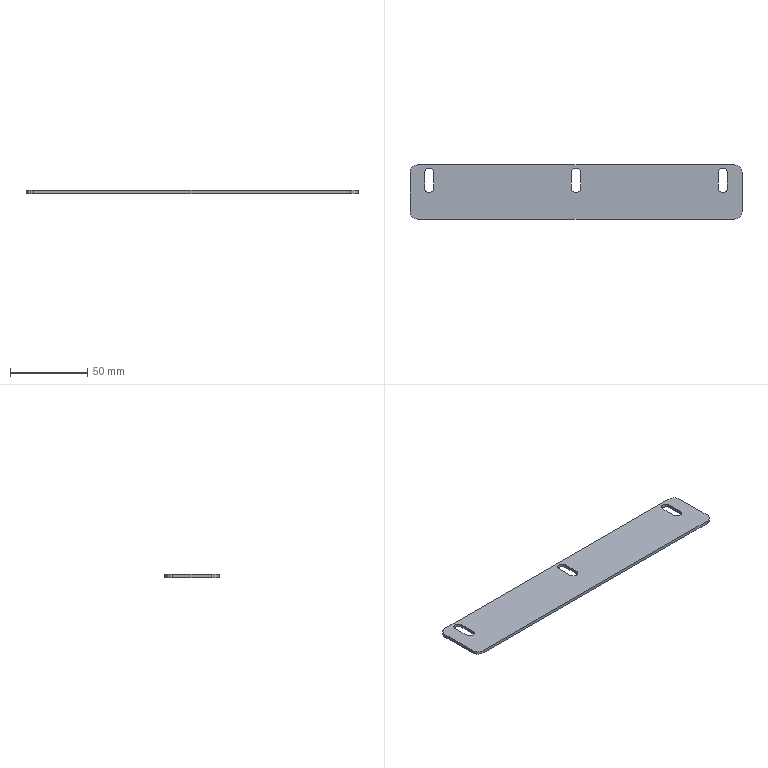Part | STEP file | FHD-021-009 front baffle | 1 solid | 22 faces | box 215 x 35 x 2 mm | volume 14477 mm3 | plane 12 | cylinder 10 | commonest cylinder face diameters 6 x6 10 x4